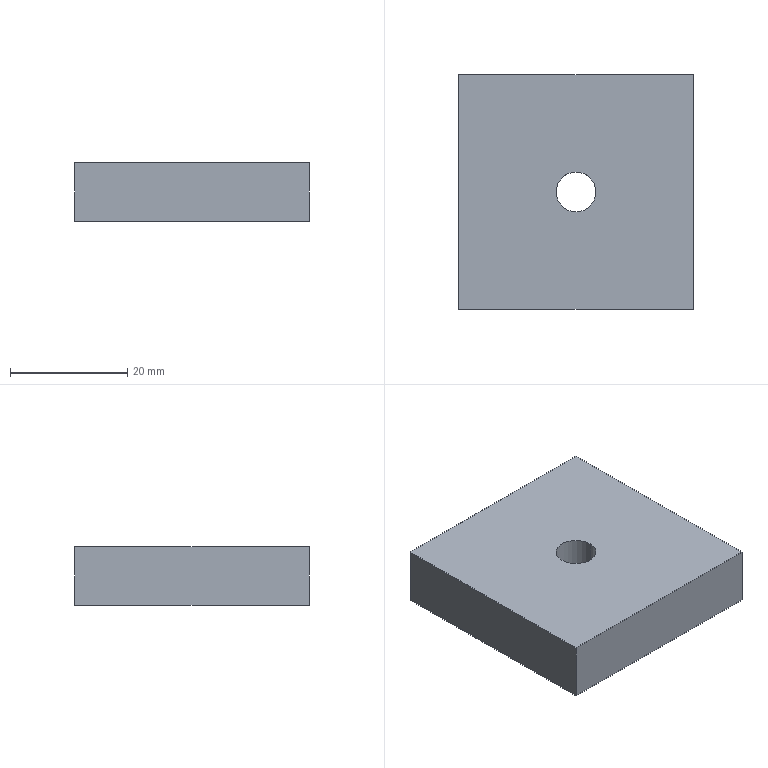Part | SolidWorks | features Extrusion 1, HoleWzd 1 | 1 solid | 8 faces | box 40 x 40 x 10 mm | volume 15637 mm3 | plane 6 | cylinder 2 | commonest cylinder face diameters 6.8 x2
STEP:
#1=CARTESIAN_POINT('',(-3.4,0.,-5.));
#2=VERTEX_POINT('',#1);
#3=CARTESIAN_POINT('',(3.4,0.,-5.));
#4=VERTEX_POINT('',#3);
#5=CARTESIAN_POINT('',(0.,0.,-5.));
#6=DIRECTION('',(0.,0.,1.));
#7=DIRECTION('',(1.,0.,0.));
#8=AXIS2_PLACEMENT_3D('',#5,#6,#7);
#9=CIRCLE('',#8,3.4);
#10=EDGE_CURVE('',#2,#4,#9,.T.);
#11=ORIENTED_EDGE('',*,*,#10,.F.);
#12=CARTESIAN_POINT('',(-3.4,0.,5.));
#13=VERTEX_POINT('',#12);
#14=CARTESIAN_POINT('',(-3.4,0.,5.));
#15=DIRECTION('',(0.,0.,1.));
#16=VECTOR('',#15,1000.);
#17=LINE('',#14,#16);
#18=EDGE_CURVE('',#2,#13,#17,.T.);
#19=ORIENTED_EDGE('',*,*,#18,.T.);
#20=CARTESIAN_POINT('',(3.4,0.,5.));
#21=VERTEX_POINT('',#20);
#22=CARTESIAN_POINT('',(0.,0.,5.));
#23=DIRECTION('',(0.,0.,1.));
#24=DIRECTION('',(1.,0.,0.));
#25=AXIS2_PLACEMENT_3D('',#22,#23,#24);
#26=CIRCLE('',#25,3.4);
#27=EDGE_CURVE('',#13,#21,#26,.T.);
#28=ORIENTED_EDGE('',*,*,#27,.T.);
#29=CARTESIAN_POINT('',(3.4,0.,5.));
#30=DIRECTION('',(0.,0.,1.));
#31=VECTOR('',#30,1000.);
#32=LINE('',#29,#31);
#33=EDGE_CURVE('',#4,#21,#32,.T.);
#34=ORIENTED_EDGE('',*,*,#33,.F.);
#35=EDGE_LOOP('',(#11,#19,#28,#34));
#36=FACE_OUTER_BOUND('',#35,.T.);
#37=CARTESIAN_POINT('',(0.,0.,5.));
#38=DIRECTION('',(0.,0.,1.));
#39=DIRECTION('',(1.,0.,0.));
#40=AXIS2_PLACEMENT_3D('',#37,#38,#39);
#41=CYLINDRICAL_SURFACE('',#40,3.4);
#42=ADVANCED_FACE('',(#36),#41,.F.);
#43=CARTESIAN_POINT('',(20.,-20.,-5.));
#44=VERTEX_POINT('',#43);
#45=CARTESIAN_POINT('',(20.,20.,-5.));
#46=VERTEX_POINT('',#45);
#47=CARTESIAN_POINT('',(20.,-20.,-5.));
#48=DIRECTION('',(0.,1.,0.));
#49=VECTOR('',#48,1000.);
#50=LINE('',#47,#49);
#51=EDGE_CURVE('',#44,#46,#50,.T.);
#52=ORIENTED_EDGE('',*,*,#51,.T.);
#53=CARTESIAN_POINT('',(20.,20.,5.));
#54=VERTEX_POINT('',#53);
#55=CARTESIAN_POINT('',(20.,20.,5.));
#56=DIRECTION('',(0.,0.,-1.));
#57=VECTOR('',#56,1000.);
#58=LINE('',#55,#57);
#59=EDGE_CURVE('',#54,#46,#58,.T.);
#60=ORIENTED_EDGE('',*,*,#59,.F.);
#61=CARTESIAN_POINT('',(20.,-20.,5.));
#62=VERTEX_POINT('',#61);
#63=CARTESIAN_POINT('',(20.,-20.,5.));
#64=DIRECTION('',(0.,1.,0.));
#65=VECTOR('',#64,1000.);
#66=LINE('',#63,#65);
#67=EDGE_CURVE('',#62,#54,#66,.T.);
#68=ORIENTED_EDGE('',*,*,#67,.F.);
#69=CARTESIAN_POINT('',(20.,-20.,5.));
#70=DIRECTION('',(0.,0.,-1.));
#71=VECTOR('',#70,1000.);
#72=LINE('',#69,#71);
#73=EDGE_CURVE('',#62,#44,#72,.T.);
#74=ORIENTED_EDGE('',*,*,#73,.T.);
#75=EDGE_LOOP('',(#52,#60,#68,#74));
#76=FACE_OUTER_BOUND('',#75,.T.);
#77=CARTESIAN_POINT('',(20.,-20.,5.));
#78=DIRECTION('',(-1.,0.,0.));
#79=DIRECTION('',(0.,0.,1.));
#80=AXIS2_PLACEMENT_3D('',#77,#78,#79);
#81=PLANE('',#80);
#82=ADVANCED_FACE('',(#76),#81,.F.);
#83=CARTESIAN_POINT('',(-20.,20.,-5.));
#84=VERTEX_POINT('',#83);
#85=CARTESIAN_POINT('',(-20.,20.,-5.));
#86=DIRECTION('',(-1.,0.,0.));
#87=VECTOR('',#86,1000.);
#88=LINE('',#85,#87);
#89=EDGE_CURVE('',#46,#84,#88,.T.);
#90=ORIENTED_EDGE('',*,*,#89,.T.);
#91=CARTESIAN_POINT('',(-20.,20.,5.));
#92=VERTEX_POINT('',#91);
#93=CARTESIAN_POINT('',(-20.,20.,5.));
#94=DIRECTION('',(0.,0.,-1.));
#95=VECTOR('',#94,1000.);
#96=LINE('',#93,#95);
#97=EDGE_CURVE('',#92,#84,#96,.T.);
#98=ORIENTED_EDGE('',*,*,#97,.F.);
#99=CARTESIAN_POINT('',(-20.,20.,5.));
#100=DIRECTION('',(-1.,0.,0.));
#101=VECTOR('',#100,1000.);
#102=LINE('',#99,#101);
#103=EDGE_CURVE('',#54,#92,#102,.T.);
#104=ORIENTED_EDGE('',*,*,#103,.F.);
#105=ORIENTED_EDGE('',*,*,#59,.T.);
#106=EDGE_LOOP('',(#90,#98,#104,#105));
#107=FACE_OUTER_BOUND('',#106,.T.);
#108=CARTESIAN_POINT('',(-20.,20.,5.));
#109=DIRECTION('',(0.,-1.,0.));
#110=DIRECTION('',(0.,0.,-1.));
#111=AXIS2_PLACEMENT_3D('',#108,#109,#110);
#112=PLANE('',#111);
#113=ADVANCED_FACE('',(#107),#112,.F.);
#114=CARTESIAN_POINT('',(-20.,-20.,-5.));
#115=VERTEX_POINT('',#114);
#116=CARTESIAN_POINT('',(-20.,-20.,-5.));
#117=DIRECTION('',(0.,-1.,0.));
#118=VECTOR('',#117,1000.);
#119=LINE('',#116,#118);
#120=EDGE_CURVE('',#84,#115,#119,.T.);
#121=ORIENTED_EDGE('',*,*,#120,.T.);
#122=CARTESIAN_POINT('',(-20.,-20.,5.));
#123=VERTEX_POINT('',#122);
#124=CARTESIAN_POINT('',(-20.,-20.,5.));
#125=DIRECTION('',(0.,0.,-1.));
#126=VECTOR('',#125,1000.);
#127=LINE('',#124,#126);
#128=EDGE_CURVE('',#123,#115,#127,.T.);
#129=ORIENTED_EDGE('',*,*,#128,.F.);
#130=CARTESIAN_POINT('',(-20.,-20.,5.));
#131=DIRECTION('',(0.,-1.,0.));
#132=VECTOR('',#131,1000.);
#133=LINE('',#130,#132);
#134=EDGE_CURVE('',#92,#123,#133,.T.);
#135=ORIENTED_EDGE('',*,*,#134,.F.);
#136=ORIENTED_EDGE('',*,*,#97,.T.);
#137=EDGE_LOOP('',(#121,#129,#135,#136));
#138=FACE_OUTER_BOUND('',#137,.T.);
#139=CARTESIAN_POINT('',(-20.,-20.,5.));
#140=DIRECTION('',(1.,0.,0.));
#141=DIRECTION('',(0.,0.,-1.));
#142=AXIS2_PLACEMENT_3D('',#139,#140,#141);
#143=PLANE('',#142);
#144=ADVANCED_FACE('',(#138),#143,.F.);
#145=CARTESIAN_POINT('',(-20.,-20.,-5.));
#146=DIRECTION('',(1.,0.,0.));
#147=VECTOR('',#146,1000.);
#148=LINE('',#145,#147);
#149=EDGE_CURVE('',#115,#44,#148,.T.);
#150=ORIENTED_EDGE('',*,*,#149,.T.);
#151=ORIENTED_EDGE('',*,*,#73,.F.);
#152=CARTESIAN_POINT('',(-20.,-20.,5.));
#153=DIRECTION('',(1.,0.,0.));
#154=VECTOR('',#153,1000.);
#155=LINE('',#152,#154);
#156=EDGE_CURVE('',#123,#62,#155,.T.);
#157=ORIENTED_EDGE('',*,*,#156,.F.);
#158=ORIENTED_EDGE('',*,*,#128,.T.);
#159=EDGE_LOOP('',(#150,#151,#157,#158));
#160=FACE_OUTER_BOUND('',#159,.T.);
#161=CARTESIAN_POINT('',(-20.,-20.,5.));
#162=DIRECTION('',(0.,1.,0.));
#163=DIRECTION('',(0.,0.,1.));
#164=AXIS2_PLACEMENT_3D('',#161,#162,#163);
#165=PLANE('',#164);
#166=ADVANCED_FACE('',(#160),#165,.F.);
#167=CARTESIAN_POINT('',(0.,0.,5.));
#168=DIRECTION('',(0.,0.,1.));
#169=DIRECTION('',(1.,0.,0.));
#170=AXIS2_PLACEMENT_3D('',#167,#168,#169);
#171=CIRCLE('',#170,3.4);
#172=EDGE_CURVE('',#21,#13,#171,.T.);
#173=ORIENTED_EDGE('',*,*,#172,.F.);
#174=ORIENTED_EDGE('',*,*,#27,.F.);
#175=EDGE_LOOP('',(#173,#174));
#176=FACE_BOUND('',#175,.T.);
#177=ORIENTED_EDGE('',*,*,#67,.T.);
#178=ORIENTED_EDGE('',*,*,#103,.T.);
#179=ORIENTED_EDGE('',*,*,#134,.T.);
#180=ORIENTED_EDGE('',*,*,#156,.T.);
#181=EDGE_LOOP('',(#177,#178,#179,#180));
#182=FACE_OUTER_BOUND('',#181,.T.);
#183=CARTESIAN_POINT('',(0.,0.,5.));
#184=DIRECTION('',(0.,0.,-1.));
#185=DIRECTION('',(-1.,0.,0.));
#186=AXIS2_PLACEMENT_3D('',#183,#184,#185);
#187=PLANE('',#186);
#188=ADVANCED_FACE('',(#176,#182),#187,.F.);
#189=CARTESIAN_POINT('',(0.,0.,-5.));
#190=DIRECTION('',(0.,0.,1.));
#191=DIRECTION('',(1.,0.,0.));
#192=AXIS2_PLACEMENT_3D('',#189,#190,#191);
#193=CIRCLE('',#192,3.4);
#194=EDGE_CURVE('',#4,#2,#193,.T.);
#195=ORIENTED_EDGE('',*,*,#194,.T.);
#196=ORIENTED_EDGE('',*,*,#10,.T.);
#197=EDGE_LOOP('',(#195,#196));
#198=FACE_BOUND('',#197,.T.);
#199=ORIENTED_EDGE('',*,*,#51,.F.);
#200=ORIENTED_EDGE('',*,*,#149,.F.);
#201=ORIENTED_EDGE('',*,*,#120,.F.);
#202=ORIENTED_EDGE('',*,*,#89,.F.);
#203=EDGE_LOOP('',(#199,#200,#201,#202));
#204=FACE_OUTER_BOUND('',#203,.T.);
#205=CARTESIAN_POINT('',(0.,0.,-5.));
#206=DIRECTION('',(0.,0.,-1.));
#207=DIRECTION('',(-1.,0.,0.));
#208=AXIS2_PLACEMENT_3D('',#205,#206,#207);
#209=PLANE('',#208);
#210=ADVANCED_FACE('',(#198,#204),#209,.T.);
#211=ORIENTED_EDGE('',*,*,#18,.F.);
#212=ORIENTED_EDGE('',*,*,#194,.F.);
#213=ORIENTED_EDGE('',*,*,#33,.T.);
#214=ORIENTED_EDGE('',*,*,#172,.T.);
#215=EDGE_LOOP('',(#211,#212,#213,#214));
#216=FACE_OUTER_BOUND('',#215,.T.);
#217=CARTESIAN_POINT('',(0.,0.,5.));
#218=DIRECTION('',(0.,0.,1.));
#219=DIRECTION('',(1.,0.,0.));
#220=AXIS2_PLACEMENT_3D('',#217,#218,#219);
#221=CYLINDRICAL_SURFACE('',#220,3.4);
#222=ADVANCED_FACE('',(#216),#221,.F.);
#223=CLOSED_SHELL('',(#42,#82,#113,#144,#166,#188,#210,#222));
#224=MANIFOLD_SOLID_BREP('',#223);
#225=CARTESIAN_POINT('',(0.,0.,0.));
#226=DIRECTION('',(0.,0.,1.));
#227=DIRECTION('',(1.,0.,0.));
#228=AXIS2_PLACEMENT_3D('',#225,#226,#227);
#229=(LENGTH_UNIT()NAMED_UNIT(*)SI_UNIT(.MILLI.,.METRE.));
#230=UNCERTAINTY_MEASURE_WITH_UNIT(LENGTH_MEASURE(0.00001),#229,'','');
#231=(NAMED_UNIT(*)PLANE_ANGLE_UNIT()SI_UNIT($,.RADIAN.));
#232=(NAMED_UNIT(*)SI_UNIT($,.STERADIAN.)SOLID_ANGLE_UNIT());
#233=(GEOMETRIC_REPRESENTATION_CONTEXT(3)GLOBAL_UNCERTAINTY_ASSIGNED_CONTEXT((#230))GLOBAL_UNIT_ASSIGNED_CONTEXT((#229,#231,#232))REPRESENTATION_CONTEXT('',''));
#234=ADVANCED_BREP_SHAPE_REPRESENTATION('',(#224,#228),#233);